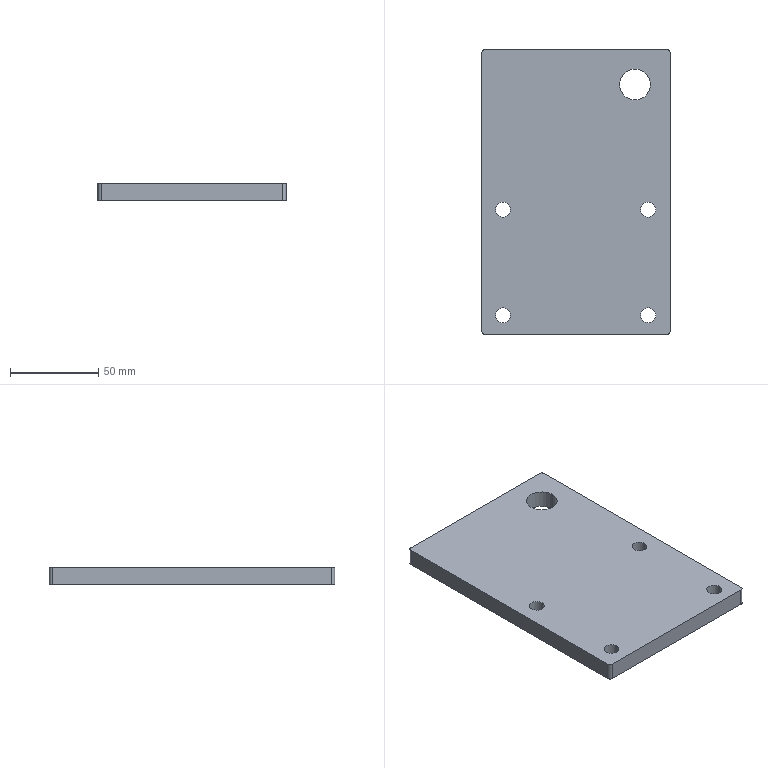Part | SolidWorks | features HoleWzd 2, Extrusion 1, Fillet 1, LPattern 1 | 1 solid | 20 faces | box 107 x 162 x 10 mm | volume 168631 mm3 | cylinder 14 | plane 6 | commonest cylinder face diameters 8.5 x8 4 x4 17.5 x2
STEP:
#1=CARTESIAN_POINT('',(36.75,-70.,-5.));
#2=VERTEX_POINT('',#1);
#3=CARTESIAN_POINT('',(45.25,-70.,-5.));
#4=VERTEX_POINT('',#3);
#5=CARTESIAN_POINT('',(41.,-70.,-5.));
#6=DIRECTION('',(0.,0.,1.));
#7=DIRECTION('',(1.,0.,0.));
#8=AXIS2_PLACEMENT_3D('',#5,#6,#7);
#9=CIRCLE('',#8,4.25);
#10=EDGE_CURVE('',#2,#4,#9,.T.);
#11=ORIENTED_EDGE('',*,*,#10,.F.);
#12=CARTESIAN_POINT('',(36.75,-70.,5.));
#13=VERTEX_POINT('',#12);
#14=CARTESIAN_POINT('',(36.75,-70.,5.));
#15=DIRECTION('',(0.,0.,1.));
#16=VECTOR('',#15,1000.);
#17=LINE('',#14,#16);
#18=EDGE_CURVE('',#2,#13,#17,.T.);
#19=ORIENTED_EDGE('',*,*,#18,.T.);
#20=CARTESIAN_POINT('',(45.25,-70.,5.));
#21=VERTEX_POINT('',#20);
#22=CARTESIAN_POINT('',(41.,-70.,5.));
#23=DIRECTION('',(0.,0.,1.));
#24=DIRECTION('',(1.,0.,0.));
#25=AXIS2_PLACEMENT_3D('',#22,#23,#24);
#26=CIRCLE('',#25,4.25);
#27=EDGE_CURVE('',#13,#21,#26,.T.);
#28=ORIENTED_EDGE('',*,*,#27,.T.);
#29=CARTESIAN_POINT('',(45.25,-70.,5.));
#30=DIRECTION('',(0.,0.,1.));
#31=VECTOR('',#30,1000.);
#32=LINE('',#29,#31);
#33=EDGE_CURVE('',#4,#21,#32,.T.);
#34=ORIENTED_EDGE('',*,*,#33,.F.);
#35=EDGE_LOOP('',(#11,#19,#28,#34));
#36=FACE_OUTER_BOUND('',#35,.T.);
#37=CARTESIAN_POINT('',(41.,-70.,5.));
#38=DIRECTION('',(0.,0.,1.));
#39=DIRECTION('',(1.,0.,0.));
#40=AXIS2_PLACEMENT_3D('',#37,#38,#39);
#41=CYLINDRICAL_SURFACE('',#40,4.25);
#42=ADVANCED_FACE('',(#36),#41,.F.);
#43=CARTESIAN_POINT('',(-45.75,-70.,-5.));
#44=VERTEX_POINT('',#43);
#45=CARTESIAN_POINT('',(-37.25,-70.,-5.));
#46=VERTEX_POINT('',#45);
#47=CARTESIAN_POINT('',(-41.5,-70.,-5.));
#48=DIRECTION('',(0.,0.,1.));
#49=DIRECTION('',(1.,0.,0.));
#50=AXIS2_PLACEMENT_3D('',#47,#48,#49);
#51=CIRCLE('',#50,4.25);
#52=EDGE_CURVE('',#44,#46,#51,.T.);
#53=ORIENTED_EDGE('',*,*,#52,.F.);
#54=CARTESIAN_POINT('',(-45.75,-70.,5.));
#55=VERTEX_POINT('',#54);
#56=CARTESIAN_POINT('',(-45.75,-70.,5.));
#57=DIRECTION('',(0.,0.,1.));
#58=VECTOR('',#57,1000.);
#59=LINE('',#56,#58);
#60=EDGE_CURVE('',#44,#55,#59,.T.);
#61=ORIENTED_EDGE('',*,*,#60,.T.);
#62=CARTESIAN_POINT('',(-37.25,-70.,5.));
#63=VERTEX_POINT('',#62);
#64=CARTESIAN_POINT('',(-41.5,-70.,5.));
#65=DIRECTION('',(0.,0.,1.));
#66=DIRECTION('',(1.,0.,0.));
#67=AXIS2_PLACEMENT_3D('',#64,#65,#66);
#68=CIRCLE('',#67,4.25);
#69=EDGE_CURVE('',#55,#63,#68,.T.);
#70=ORIENTED_EDGE('',*,*,#69,.T.);
#71=CARTESIAN_POINT('',(-37.25,-70.,5.));
#72=DIRECTION('',(0.,0.,1.));
#73=VECTOR('',#72,1000.);
#74=LINE('',#71,#73);
#75=EDGE_CURVE('',#46,#63,#74,.T.);
#76=ORIENTED_EDGE('',*,*,#75,.F.);
#77=EDGE_LOOP('',(#53,#61,#70,#76));
#78=FACE_OUTER_BOUND('',#77,.T.);
#79=CARTESIAN_POINT('',(-41.5,-70.,5.));
#80=DIRECTION('',(0.,0.,1.));
#81=DIRECTION('',(1.,0.,0.));
#82=AXIS2_PLACEMENT_3D('',#79,#80,#81);
#83=CYLINDRICAL_SURFACE('',#82,4.25);
#84=ADVANCED_FACE('',(#78),#83,.F.);
#85=CARTESIAN_POINT('',(24.75,61.,-5.));
#86=VERTEX_POINT('',#85);
#87=CARTESIAN_POINT('',(42.25,61.,-5.));
#88=VERTEX_POINT('',#87);
#89=CARTESIAN_POINT('',(33.5,61.,-5.));
#90=DIRECTION('',(0.,0.,1.));
#91=DIRECTION('',(1.,0.,0.));
#92=AXIS2_PLACEMENT_3D('',#89,#90,#91);
#93=CIRCLE('',#92,8.75);
#94=EDGE_CURVE('',#86,#88,#93,.T.);
#95=ORIENTED_EDGE('',*,*,#94,.F.);
#96=CARTESIAN_POINT('',(24.75,61.,5.));
#97=VERTEX_POINT('',#96);
#98=CARTESIAN_POINT('',(24.75,61.,5.));
#99=DIRECTION('',(0.,0.,1.));
#100=VECTOR('',#99,1000.);
#101=LINE('',#98,#100);
#102=EDGE_CURVE('',#86,#97,#101,.T.);
#103=ORIENTED_EDGE('',*,*,#102,.T.);
#104=CARTESIAN_POINT('',(42.25,61.,5.));
#105=VERTEX_POINT('',#104);
#106=CARTESIAN_POINT('',(33.5,61.,5.));
#107=DIRECTION('',(0.,0.,1.));
#108=DIRECTION('',(1.,0.,0.));
#109=AXIS2_PLACEMENT_3D('',#106,#107,#108);
#110=CIRCLE('',#109,8.75);
#111=EDGE_CURVE('',#97,#105,#110,.T.);
#112=ORIENTED_EDGE('',*,*,#111,.T.);
#113=CARTESIAN_POINT('',(42.25,61.,5.));
#114=DIRECTION('',(0.,0.,1.));
#115=VECTOR('',#114,1000.);
#116=LINE('',#113,#115);
#117=EDGE_CURVE('',#88,#105,#116,.T.);
#118=ORIENTED_EDGE('',*,*,#117,.F.);
#119=EDGE_LOOP('',(#95,#103,#112,#118));
#120=FACE_OUTER_BOUND('',#119,.T.);
#121=CARTESIAN_POINT('',(33.5,61.,5.));
#122=DIRECTION('',(0.,0.,1.));
#123=DIRECTION('',(1.,0.,0.));
#124=AXIS2_PLACEMENT_3D('',#121,#122,#123);
#125=CYLINDRICAL_SURFACE('',#124,8.75);
#126=ADVANCED_FACE('',(#120),#125,.F.);
#127=CARTESIAN_POINT('',(-45.75,-10.,-5.));
#128=VERTEX_POINT('',#127);
#129=CARTESIAN_POINT('',(-37.25,-10.,-5.));
#130=VERTEX_POINT('',#129);
#131=CARTESIAN_POINT('',(-41.5,-10.,-5.));
#132=DIRECTION('',(0.,0.,1.));
#133=DIRECTION('',(1.,0.,0.));
#134=AXIS2_PLACEMENT_3D('',#131,#132,#133);
#135=CIRCLE('',#134,4.25);
#136=EDGE_CURVE('',#128,#130,#135,.T.);
#137=ORIENTED_EDGE('',*,*,#136,.F.);
#138=CARTESIAN_POINT('',(-45.75,-10.,5.));
#139=VERTEX_POINT('',#138);
#140=CARTESIAN_POINT('',(-45.75,-10.,5.));
#141=DIRECTION('',(0.,0.,1.));
#142=VECTOR('',#141,1000.);
#143=LINE('',#140,#142);
#144=EDGE_CURVE('',#128,#139,#143,.T.);
#145=ORIENTED_EDGE('',*,*,#144,.T.);
#146=CARTESIAN_POINT('',(-37.25,-10.,5.));
#147=VERTEX_POINT('',#146);
#148=CARTESIAN_POINT('',(-41.5,-10.,5.));
#149=DIRECTION('',(0.,0.,1.));
#150=DIRECTION('',(1.,0.,0.));
#151=AXIS2_PLACEMENT_3D('',#148,#149,#150);
#152=CIRCLE('',#151,4.25);
#153=EDGE_CURVE('',#139,#147,#152,.T.);
#154=ORIENTED_EDGE('',*,*,#153,.T.);
#155=CARTESIAN_POINT('',(-37.25,-10.,5.));
#156=DIRECTION('',(0.,0.,1.));
#157=VECTOR('',#156,1000.);
#158=LINE('',#155,#157);
#159=EDGE_CURVE('',#130,#147,#158,.T.);
#160=ORIENTED_EDGE('',*,*,#159,.F.);
#161=EDGE_LOOP('',(#137,#145,#154,#160));
#162=FACE_OUTER_BOUND('',#161,.T.);
#163=CARTESIAN_POINT('',(-41.5,-10.,5.));
#164=DIRECTION('',(0.,0.,1.));
#165=DIRECTION('',(1.,0.,0.));
#166=AXIS2_PLACEMENT_3D('',#163,#164,#165);
#167=CYLINDRICAL_SURFACE('',#166,4.25);
#168=ADVANCED_FACE('',(#162),#167,.F.);
#169=CARTESIAN_POINT('',(36.75,-10.,-5.));
#170=VERTEX_POINT('',#169);
#171=CARTESIAN_POINT('',(45.25,-10.,-5.));
#172=VERTEX_POINT('',#171);
#173=CARTESIAN_POINT('',(41.,-10.,-5.));
#174=DIRECTION('',(0.,0.,1.));
#175=DIRECTION('',(1.,0.,0.));
#176=AXIS2_PLACEMENT_3D('',#173,#174,#175);
#177=CIRCLE('',#176,4.25);
#178=EDGE_CURVE('',#170,#172,#177,.T.);
#179=ORIENTED_EDGE('',*,*,#178,.F.);
#180=CARTESIAN_POINT('',(36.75,-10.,5.));
#181=VERTEX_POINT('',#180);
#182=CARTESIAN_POINT('',(36.75,-10.,5.));
#183=DIRECTION('',(0.,0.,1.));
#184=VECTOR('',#183,1000.);
#185=LINE('',#182,#184);
#186=EDGE_CURVE('',#170,#181,#185,.T.);
#187=ORIENTED_EDGE('',*,*,#186,.T.);
#188=CARTESIAN_POINT('',(45.25,-10.,5.));
#189=VERTEX_POINT('',#188);
#190=CARTESIAN_POINT('',(41.,-10.,5.));
#191=DIRECTION('',(0.,0.,1.));
#192=DIRECTION('',(1.,0.,0.));
#193=AXIS2_PLACEMENT_3D('',#190,#191,#192);
#194=CIRCLE('',#193,4.25);
#195=EDGE_CURVE('',#181,#189,#194,.T.);
#196=ORIENTED_EDGE('',*,*,#195,.T.);
#197=CARTESIAN_POINT('',(45.25,-10.,5.));
#198=DIRECTION('',(0.,0.,1.));
#199=VECTOR('',#198,1000.);
#200=LINE('',#197,#199);
#201=EDGE_CURVE('',#172,#189,#200,.T.);
#202=ORIENTED_EDGE('',*,*,#201,.F.);
#203=EDGE_LOOP('',(#179,#187,#196,#202));
#204=FACE_OUTER_BOUND('',#203,.T.);
#205=CARTESIAN_POINT('',(41.,-10.,5.));
#206=DIRECTION('',(0.,0.,1.));
#207=DIRECTION('',(1.,0.,0.));
#208=AXIS2_PLACEMENT_3D('',#205,#206,#207);
#209=CYLINDRICAL_SURFACE('',#208,4.25);
#210=ADVANCED_FACE('',(#204),#209,.F.);
#211=ORIENTED_EDGE('',*,*,#186,.F.);
#212=CARTESIAN_POINT('',(41.,-10.,-5.));
#213=DIRECTION('',(0.,0.,1.));
#214=DIRECTION('',(1.,0.,0.));
#215=AXIS2_PLACEMENT_3D('',#212,#213,#214);
#216=CIRCLE('',#215,4.25);
#217=EDGE_CURVE('',#172,#170,#216,.T.);
#218=ORIENTED_EDGE('',*,*,#217,.F.);
#219=ORIENTED_EDGE('',*,*,#201,.T.);
#220=CARTESIAN_POINT('',(41.,-10.,5.));
#221=DIRECTION('',(0.,0.,1.));
#222=DIRECTION('',(1.,0.,0.));
#223=AXIS2_PLACEMENT_3D('',#220,#221,#222);
#224=CIRCLE('',#223,4.25);
#225=EDGE_CURVE('',#189,#181,#224,.T.);
#226=ORIENTED_EDGE('',*,*,#225,.T.);
#227=EDGE_LOOP('',(#211,#218,#219,#226));
#228=FACE_OUTER_BOUND('',#227,.T.);
#229=CARTESIAN_POINT('',(41.,-10.,5.));
#230=DIRECTION('',(0.,0.,1.));
#231=DIRECTION('',(1.,0.,0.));
#232=AXIS2_PLACEMENT_3D('',#229,#230,#231);
#233=CYLINDRICAL_SURFACE('',#232,4.25);
#234=ADVANCED_FACE('',(#228),#233,.F.);
#235=ORIENTED_EDGE('',*,*,#144,.F.);
#236=CARTESIAN_POINT('',(-41.5,-10.,-5.));
#237=DIRECTION('',(0.,0.,1.));
#238=DIRECTION('',(1.,0.,0.));
#239=AXIS2_PLACEMENT_3D('',#236,#237,#238);
#240=CIRCLE('',#239,4.25);
#241=EDGE_CURVE('',#130,#128,#240,.T.);
#242=ORIENTED_EDGE('',*,*,#241,.F.);
#243=ORIENTED_EDGE('',*,*,#159,.T.);
#244=CARTESIAN_POINT('',(-41.5,-10.,5.));
#245=DIRECTION('',(0.,0.,1.));
#246=DIRECTION('',(1.,0.,0.));
#247=AXIS2_PLACEMENT_3D('',#244,#245,#246);
#248=CIRCLE('',#247,4.25);
#249=EDGE_CURVE('',#147,#139,#248,.T.);
#250=ORIENTED_EDGE('',*,*,#249,.T.);
#251=EDGE_LOOP('',(#235,#242,#243,#250));
#252=FACE_OUTER_BOUND('',#251,.T.);
#253=CARTESIAN_POINT('',(-41.5,-10.,5.));
#254=DIRECTION('',(0.,0.,1.));
#255=DIRECTION('',(1.,0.,0.));
#256=AXIS2_PLACEMENT_3D('',#253,#254,#255);
#257=CYLINDRICAL_SURFACE('',#256,4.25);
#258=ADVANCED_FACE('',(#252),#257,.F.);
#259=CARTESIAN_POINT('',(41.,-70.,-5.));
#260=DIRECTION('',(0.,0.,1.));
#261=DIRECTION('',(1.,0.,0.));
#262=AXIS2_PLACEMENT_3D('',#259,#260,#261);
#263=CIRCLE('',#262,4.25);
#264=EDGE_CURVE('',#4,#2,#263,.T.);
#265=ORIENTED_EDGE('',*,*,#264,.T.);
#266=ORIENTED_EDGE('',*,*,#10,.T.);
#267=EDGE_LOOP('',(#265,#266));
#268=FACE_BOUND('',#267,.T.);
#269=CARTESIAN_POINT('',(-51.5,-81.,-5.));
#270=VERTEX_POINT('',#269);
#271=CARTESIAN_POINT('',(51.5,-81.,-5.));
#272=VERTEX_POINT('',#271);
#273=CARTESIAN_POINT('',(-53.5,-81.,-5.));
#274=DIRECTION('',(1.,0.,0.));
#275=VECTOR('',#274,1000.);
#276=LINE('',#273,#275);
#277=EDGE_CURVE('',#270,#272,#276,.T.);
#278=ORIENTED_EDGE('',*,*,#277,.F.);
#279=CARTESIAN_POINT('',(-53.5,-79.,-5.));
#280=VERTEX_POINT('',#279);
#281=CARTESIAN_POINT('',(-51.5,-79.,-5.));
#282=DIRECTION('',(0.,0.,-1.));
#283=DIRECTION('',(-1.,0.,0.));
#284=AXIS2_PLACEMENT_3D('',#281,#282,#283);
#285=CIRCLE('',#284,2.);
#286=EDGE_CURVE('',#270,#280,#285,.T.);
#287=ORIENTED_EDGE('',*,*,#286,.T.);
#288=CARTESIAN_POINT('',(-53.5,79.,-5.));
#289=VERTEX_POINT('',#288);
#290=CARTESIAN_POINT('',(-53.5,-81.,-5.));
#291=DIRECTION('',(0.,-1.,0.));
#292=VECTOR('',#291,1000.);
#293=LINE('',#290,#292);
#294=EDGE_CURVE('',#289,#280,#293,.T.);
#295=ORIENTED_EDGE('',*,*,#294,.F.);
#296=CARTESIAN_POINT('',(-51.5,81.,-5.));
#297=VERTEX_POINT('',#296);
#298=CARTESIAN_POINT('',(-51.5,79.,-5.));
#299=DIRECTION('',(0.,0.,-1.));
#300=DIRECTION('',(-1.,0.,0.));
#301=AXIS2_PLACEMENT_3D('',#298,#299,#300);
#302=CIRCLE('',#301,2.);
#303=EDGE_CURVE('',#289,#297,#302,.T.);
#304=ORIENTED_EDGE('',*,*,#303,.T.);
#305=CARTESIAN_POINT('',(51.5,81.,-5.));
#306=VERTEX_POINT('',#305);
#307=CARTESIAN_POINT('',(-53.5,81.,-5.));
#308=DIRECTION('',(-1.,0.,0.));
#309=VECTOR('',#308,1000.);
#310=LINE('',#307,#309);
#311=EDGE_CURVE('',#306,#297,#310,.T.);
#312=ORIENTED_EDGE('',*,*,#311,.F.);
#313=CARTESIAN_POINT('',(53.5,79.,-5.));
#314=VERTEX_POINT('',#313);
#315=CARTESIAN_POINT('',(51.5,79.,-5.));
#316=DIRECTION('',(0.,0.,-1.));
#317=DIRECTION('',(-1.,0.,0.));
#318=AXIS2_PLACEMENT_3D('',#315,#316,#317);
#319=CIRCLE('',#318,2.);
#320=EDGE_CURVE('',#306,#314,#319,.T.);
#321=ORIENTED_EDGE('',*,*,#320,.T.);
#322=CARTESIAN_POINT('',(53.5,-79.,-5.));
#323=VERTEX_POINT('',#322);
#324=CARTESIAN_POINT('',(53.5,-81.,-5.));
#325=DIRECTION('',(0.,1.,0.));
#326=VECTOR('',#325,1000.);
#327=LINE('',#324,#326);
#328=EDGE_CURVE('',#323,#314,#327,.T.);
#329=ORIENTED_EDGE('',*,*,#328,.F.);
#330=CARTESIAN_POINT('',(51.5,-79.,-5.));
#331=DIRECTION('',(0.,0.,-1.));
#332=DIRECTION('',(-1.,0.,0.));
#333=AXIS2_PLACEMENT_3D('',#330,#331,#332);
#334=CIRCLE('',#333,2.);
#335=EDGE_CURVE('',#323,#272,#334,.T.);
#336=ORIENTED_EDGE('',*,*,#335,.T.);
#337=EDGE_LOOP('',(#278,#287,#295,#304,#312,#321,#329,#336));
#338=FACE_OUTER_BOUND('',#337,.T.);
#339=CARTESIAN_POINT('',(33.5,61.,-5.));
#340=DIRECTION('',(0.,0.,1.));
#341=DIRECTION('',(1.,0.,0.));
#342=AXIS2_PLACEMENT_3D('',#339,#340,#341);
#343=CIRCLE('',#342,8.75);
#344=EDGE_CURVE('',#88,#86,#343,.T.);
#345=ORIENTED_EDGE('',*,*,#344,.T.);
#346=ORIENTED_EDGE('',*,*,#94,.T.);
#347=EDGE_LOOP('',(#345,#346));
#348=FACE_BOUND('',#347,.T.);
#349=CARTESIAN_POINT('',(-41.5,-70.,-5.));
#350=DIRECTION('',(0.,0.,1.));
#351=DIRECTION('',(1.,0.,0.));
#352=AXIS2_PLACEMENT_3D('',#349,#350,#351);
#353=CIRCLE('',#352,4.25);
#354=EDGE_CURVE('',#46,#44,#353,.T.);
#355=ORIENTED_EDGE('',*,*,#354,.T.);
#356=ORIENTED_EDGE('',*,*,#52,.T.);
#357=EDGE_LOOP('',(#355,#356));
#358=FACE_BOUND('',#357,.T.);
#359=ORIENTED_EDGE('',*,*,#241,.T.);
#360=ORIENTED_EDGE('',*,*,#136,.T.);
#361=EDGE_LOOP('',(#359,#360));
#362=FACE_BOUND('',#361,.T.);
#363=ORIENTED_EDGE('',*,*,#217,.T.);
#364=ORIENTED_EDGE('',*,*,#178,.T.);
#365=EDGE_LOOP('',(#363,#364));
#366=FACE_BOUND('',#365,.T.);
#367=CARTESIAN_POINT('',(0.,0.,-5.));
#368=DIRECTION('',(0.,0.,-1.));
#369=DIRECTION('',(-1.,0.,0.));
#370=AXIS2_PLACEMENT_3D('',#367,#368,#369);
#371=PLANE('',#370);
#372=ADVANCED_FACE('',(#268,#338,#348,#358,#362,#366),#371,.T.);
#373=CARTESIAN_POINT('',(53.5,-79.,5.));
#374=VERTEX_POINT('',#373);
#375=CARTESIAN_POINT('',(53.5,79.,5.));
#376=VERTEX_POINT('',#375);
#377=CARTESIAN_POINT('',(53.5,-81.,5.));
#378=DIRECTION('',(0.,1.,0.));
#379=VECTOR('',#378,1000.);
#380=LINE('',#377,#379);
#381=EDGE_CURVE('',#374,#376,#380,.T.);
#382=ORIENTED_EDGE('',*,*,#381,.F.);
#383=CARTESIAN_POINT('',(53.5,-79.,5.));
#384=DIRECTION('',(0.,0.,-1.));
#385=VECTOR('',#384,1000.);
#386=LINE('',#383,#385);
#387=EDGE_CURVE('',#374,#323,#386,.T.);
#388=ORIENTED_EDGE('',*,*,#387,.T.);
#389=ORIENTED_EDGE('',*,*,#328,.T.);
#390=CARTESIAN_POINT('',(53.5,79.,5.));
#391=DIRECTION('',(0.,0.,1.));
#392=VECTOR('',#391,1000.);
#393=LINE('',#390,#392);
#394=EDGE_CURVE('',#314,#376,#393,.T.);
#395=ORIENTED_EDGE('',*,*,#394,.T.);
#396=EDGE_LOOP('',(#382,#388,#389,#395));
#397=FACE_OUTER_BOUND('',#396,.T.);
#398=CARTESIAN_POINT('',(53.5,-81.,5.));
#399=DIRECTION('',(-1.,0.,0.));
#400=DIRECTION('',(0.,0.,1.));
#401=AXIS2_PLACEMENT_3D('',#398,#399,#400);
#402=PLANE('',#401);
#403=ADVANCED_FACE('',(#397),#402,.F.);
#404=CARTESIAN_POINT('',(51.5,81.,5.));
#405=VERTEX_POINT('',#404);
#406=CARTESIAN_POINT('',(-51.5,81.,5.));
#407=VERTEX_POINT('',#406);
#408=CARTESIAN_POINT('',(-53.5,81.,5.));
#409=DIRECTION('',(-1.,0.,0.));
#410=VECTOR('',#409,1000.);
#411=LINE('',#408,#410);
#412=EDGE_CURVE('',#405,#407,#411,.T.);
#413=ORIENTED_EDGE('',*,*,#412,.F.);
#414=CARTESIAN_POINT('',(51.5,81.,5.));
#415=DIRECTION('',(0.,0.,-1.));
#416=VECTOR('',#415,1000.);
#417=LINE('',#414,#416);
#418=EDGE_CURVE('',#405,#306,#417,.T.);
#419=ORIENTED_EDGE('',*,*,#418,.T.);
#420=ORIENTED_EDGE('',*,*,#311,.T.);
#421=CARTESIAN_POINT('',(-51.5,81.,5.));
#422=DIRECTION('',(0.,0.,1.));
#423=VECTOR('',#422,1000.);
#424=LINE('',#421,#423);
#425=EDGE_CURVE('',#297,#407,#424,.T.);
#426=ORIENTED_EDGE('',*,*,#425,.T.);
#427=EDGE_LOOP('',(#413,#419,#420,#426));
#428=FACE_OUTER_BOUND('',#427,.T.);
#429=CARTESIAN_POINT('',(-53.5,81.,5.));
#430=DIRECTION('',(0.,-1.,0.));
#431=DIRECTION('',(0.,0.,-1.));
#432=AXIS2_PLACEMENT_3D('',#429,#430,#431);
#433=PLANE('',#432);
#434=ADVANCED_FACE('',(#428),#433,.F.);
#435=ORIENTED_EDGE('',*,*,#294,.T.);
#436=CARTESIAN_POINT('',(-53.5,-79.,5.));
#437=VERTEX_POINT('',#436);
#438=CARTESIAN_POINT('',(-53.5,-79.,5.));
#439=DIRECTION('',(0.,0.,1.));
#440=VECTOR('',#439,1000.);
#441=LINE('',#438,#440);
#442=EDGE_CURVE('',#280,#437,#441,.T.);
#443=ORIENTED_EDGE('',*,*,#442,.T.);
#444=CARTESIAN_POINT('',(-53.5,79.,5.));
#445=VERTEX_POINT('',#444);
#446=CARTESIAN_POINT('',(-53.5,-81.,5.));
#447=DIRECTION('',(0.,-1.,0.));
#448=VECTOR('',#447,1000.);
#449=LINE('',#446,#448);
#450=EDGE_CURVE('',#445,#437,#449,.T.);
#451=ORIENTED_EDGE('',*,*,#450,.F.);
#452=CARTESIAN_POINT('',(-53.5,79.,5.));
#453=DIRECTION('',(0.,0.,-1.));
#454=VECTOR('',#453,1000.);
#455=LINE('',#452,#454);
#456=EDGE_CURVE('',#445,#289,#455,.T.);
#457=ORIENTED_EDGE('',*,*,#456,.T.);
#458=EDGE_LOOP('',(#435,#443,#451,#457));
#459=FACE_OUTER_BOUND('',#458,.T.);
#460=CARTESIAN_POINT('',(-53.5,-81.,5.));
#461=DIRECTION('',(1.,0.,0.));
#462=DIRECTION('',(0.,0.,-1.));
#463=AXIS2_PLACEMENT_3D('',#460,#461,#462);
#464=PLANE('',#463);
#465=ADVANCED_FACE('',(#459),#464,.F.);
#466=CARTESIAN_POINT('',(-51.5,-81.,5.));
#467=VERTEX_POINT('',#466);
#468=CARTESIAN_POINT('',(51.5,-81.,5.));
#469=VERTEX_POINT('',#468);
#470=CARTESIAN_POINT('',(-53.5,-81.,5.));
#471=DIRECTION('',(1.,0.,0.));
#472=VECTOR('',#471,1000.);
#473=LINE('',#470,#472);
#474=EDGE_CURVE('',#467,#469,#473,.T.);
#475=ORIENTED_EDGE('',*,*,#474,.F.);
#476=CARTESIAN_POINT('',(-51.5,-81.,5.));
#477=DIRECTION('',(0.,0.,-1.));
#478=VECTOR('',#477,1000.);
#479=LINE('',#476,#478);
#480=EDGE_CURVE('',#467,#270,#479,.T.);
#481=ORIENTED_EDGE('',*,*,#480,.T.);
#482=ORIENTED_EDGE('',*,*,#277,.T.);
#483=CARTESIAN_POINT('',(51.5,-81.,5.));
#484=DIRECTION('',(0.,0.,1.));
#485=VECTOR('',#484,1000.);
#486=LINE('',#483,#485);
#487=EDGE_CURVE('',#272,#469,#486,.T.);
#488=ORIENTED_EDGE('',*,*,#487,.T.);
#489=EDGE_LOOP('',(#475,#481,#482,#488));
#490=FACE_OUTER_BOUND('',#489,.T.);
#491=CARTESIAN_POINT('',(-53.5,-81.,5.));
#492=DIRECTION('',(0.,1.,0.));
#493=DIRECTION('',(0.,0.,1.));
#494=AXIS2_PLACEMENT_3D('',#491,#492,#493);
#495=PLANE('',#494);
#496=ADVANCED_FACE('',(#490),#495,.F.);
#497=CARTESIAN_POINT('',(41.,-70.,5.));
#498=DIRECTION('',(0.,0.,1.));
#499=DIRECTION('',(1.,0.,0.));
#500=AXIS2_PLACEMENT_3D('',#497,#498,#499);
#501=CIRCLE('',#500,4.25);
#502=EDGE_CURVE('',#21,#13,#501,.T.);
#503=ORIENTED_EDGE('',*,*,#502,.F.);
#504=ORIENTED_EDGE('',*,*,#27,.F.);
#505=EDGE_LOOP('',(#503,#504));
#506=FACE_BOUND('',#505,.T.);
#507=CARTESIAN_POINT('',(-41.5,-70.,5.));
#508=DIRECTION('',(0.,0.,1.));
#509=DIRECTION('',(1.,0.,0.));
#510=AXIS2_PLACEMENT_3D('',#507,#508,#509);
#511=CIRCLE('',#510,4.25);
#512=EDGE_CURVE('',#63,#55,#511,.T.);
#513=ORIENTED_EDGE('',*,*,#512,.F.);
#514=ORIENTED_EDGE('',*,*,#69,.F.);
#515=EDGE_LOOP('',(#513,#514));
#516=FACE_BOUND('',#515,.T.);
#517=CARTESIAN_POINT('',(33.5,61.,5.));
#518=DIRECTION('',(0.,0.,1.));
#519=DIRECTION('',(1.,0.,0.));
#520=AXIS2_PLACEMENT_3D('',#517,#518,#519);
#521=CIRCLE('',#520,8.75);
#522=EDGE_CURVE('',#105,#97,#521,.T.);
#523=ORIENTED_EDGE('',*,*,#522,.F.);
#524=ORIENTED_EDGE('',*,*,#111,.F.);
#525=EDGE_LOOP('',(#523,#524));
#526=FACE_BOUND('',#525,.T.);
#527=ORIENTED_EDGE('',*,*,#450,.T.);
#528=CARTESIAN_POINT('',(-51.5,-79.,5.));
#529=DIRECTION('',(0.,0.,1.));
#530=DIRECTION('',(-1.,0.,0.));
#531=AXIS2_PLACEMENT_3D('',#528,#529,#530);
#532=CIRCLE('',#531,2.);
#533=EDGE_CURVE('',#437,#467,#532,.T.);
#534=ORIENTED_EDGE('',*,*,#533,.T.);
#535=ORIENTED_EDGE('',*,*,#474,.T.);
#536=CARTESIAN_POINT('',(51.5,-79.,5.));
#537=DIRECTION('',(0.,0.,1.));
#538=DIRECTION('',(-1.,0.,0.));
#539=AXIS2_PLACEMENT_3D('',#536,#537,#538);
#540=CIRCLE('',#539,2.);
#541=EDGE_CURVE('',#469,#374,#540,.T.);
#542=ORIENTED_EDGE('',*,*,#541,.T.);
#543=ORIENTED_EDGE('',*,*,#381,.T.);
#544=CARTESIAN_POINT('',(51.5,79.,5.));
#545=DIRECTION('',(0.,0.,1.));
#546=DIRECTION('',(-1.,0.,0.));
#547=AXIS2_PLACEMENT_3D('',#544,#545,#546);
#548=CIRCLE('',#547,2.);
#549=EDGE_CURVE('',#376,#405,#548,.T.);
#550=ORIENTED_EDGE('',*,*,#549,.T.);
#551=ORIENTED_EDGE('',*,*,#412,.T.);
#552=CARTESIAN_POINT('',(-51.5,79.,5.));
#553=DIRECTION('',(0.,0.,1.));
#554=DIRECTION('',(-1.,0.,0.));
#555=AXIS2_PLACEMENT_3D('',#552,#553,#554);
#556=CIRCLE('',#555,2.);
#557=EDGE_CURVE('',#407,#445,#556,.T.);
#558=ORIENTED_EDGE('',*,*,#557,.T.);
#559=EDGE_LOOP('',(#527,#534,#535,#542,#543,#550,#551,#558));
#560=FACE_OUTER_BOUND('',#559,.T.);
#561=ORIENTED_EDGE('',*,*,#249,.F.);
#562=ORIENTED_EDGE('',*,*,#153,.F.);
#563=EDGE_LOOP('',(#561,#562));
#564=FACE_BOUND('',#563,.T.);
#565=ORIENTED_EDGE('',*,*,#225,.F.);
#566=ORIENTED_EDGE('',*,*,#195,.F.);
#567=EDGE_LOOP('',(#565,#566));
#568=FACE_BOUND('',#567,.T.);
#569=CARTESIAN_POINT('',(0.,0.,5.));
#570=DIRECTION('',(0.,0.,-1.));
#571=DIRECTION('',(-1.,0.,0.));
#572=AXIS2_PLACEMENT_3D('',#569,#570,#571);
#573=PLANE('',#572);
#574=ADVANCED_FACE('',(#506,#516,#526,#560,#564,#568),#573,.F.);
#575=ORIENTED_EDGE('',*,*,#102,.F.);
#576=ORIENTED_EDGE('',*,*,#344,.F.);
#577=ORIENTED_EDGE('',*,*,#117,.T.);
#578=ORIENTED_EDGE('',*,*,#522,.T.);
#579=EDGE_LOOP('',(#575,#576,#577,#578));
#580=FACE_OUTER_BOUND('',#579,.T.);
#581=CARTESIAN_POINT('',(33.5,61.,5.));
#582=DIRECTION('',(0.,0.,1.));
#583=DIRECTION('',(1.,0.,0.));
#584=AXIS2_PLACEMENT_3D('',#581,#582,#583);
#585=CYLINDRICAL_SURFACE('',#584,8.75);
#586=ADVANCED_FACE('',(#580),#585,.F.);
#587=ORIENTED_EDGE('',*,*,#533,.F.);
#588=ORIENTED_EDGE('',*,*,#442,.F.);
#589=ORIENTED_EDGE('',*,*,#286,.F.);
#590=ORIENTED_EDGE('',*,*,#480,.F.);
#591=EDGE_LOOP('',(#587,#588,#589,#590));
#592=FACE_OUTER_BOUND('',#591,.T.);
#593=CARTESIAN_POINT('',(-51.5,-79.,5.));
#594=DIRECTION('',(0.,0.,-1.));
#595=DIRECTION('',(-1.,0.,0.));
#596=AXIS2_PLACEMENT_3D('',#593,#594,#595);
#597=CYLINDRICAL_SURFACE('',#596,2.);
#598=ADVANCED_FACE('',(#592),#597,.T.);
#599=ORIENTED_EDGE('',*,*,#541,.F.);
#600=ORIENTED_EDGE('',*,*,#487,.F.);
#601=ORIENTED_EDGE('',*,*,#335,.F.);
#602=ORIENTED_EDGE('',*,*,#387,.F.);
#603=EDGE_LOOP('',(#599,#600,#601,#602));
#604=FACE_OUTER_BOUND('',#603,.T.);
#605=CARTESIAN_POINT('',(51.5,-79.,5.));
#606=DIRECTION('',(0.,0.,-1.));
#607=DIRECTION('',(-1.,0.,0.));
#608=AXIS2_PLACEMENT_3D('',#605,#606,#607);
#609=CYLINDRICAL_SURFACE('',#608,2.);
#610=ADVANCED_FACE('',(#604),#609,.T.);
#611=ORIENTED_EDGE('',*,*,#549,.F.);
#612=ORIENTED_EDGE('',*,*,#394,.F.);
#613=ORIENTED_EDGE('',*,*,#320,.F.);
#614=ORIENTED_EDGE('',*,*,#418,.F.);
#615=EDGE_LOOP('',(#611,#612,#613,#614));
#616=FACE_OUTER_BOUND('',#615,.T.);
#617=CARTESIAN_POINT('',(51.5,79.,5.));
#618=DIRECTION('',(0.,0.,-1.));
#619=DIRECTION('',(-1.,0.,0.));
#620=AXIS2_PLACEMENT_3D('',#617,#618,#619);
#621=CYLINDRICAL_SURFACE('',#620,2.);
#622=ADVANCED_FACE('',(#616),#621,.T.);
#623=ORIENTED_EDGE('',*,*,#557,.F.);
#624=ORIENTED_EDGE('',*,*,#425,.F.);
#625=ORIENTED_EDGE('',*,*,#303,.F.);
#626=ORIENTED_EDGE('',*,*,#456,.F.);
#627=EDGE_LOOP('',(#623,#624,#625,#626));
#628=FACE_OUTER_BOUND('',#627,.T.);
#629=CARTESIAN_POINT('',(-51.5,79.,5.));
#630=DIRECTION('',(0.,0.,-1.));
#631=DIRECTION('',(-1.,0.,0.));
#632=AXIS2_PLACEMENT_3D('',#629,#630,#631);
#633=CYLINDRICAL_SURFACE('',#632,2.);
#634=ADVANCED_FACE('',(#628),#633,.T.);
#635=ORIENTED_EDGE('',*,*,#60,.F.);
#636=ORIENTED_EDGE('',*,*,#354,.F.);
#637=ORIENTED_EDGE('',*,*,#75,.T.);
#638=ORIENTED_EDGE('',*,*,#512,.T.);
#639=EDGE_LOOP('',(#635,#636,#637,#638));
#640=FACE_OUTER_BOUND('',#639,.T.);
#641=CARTESIAN_POINT('',(-41.5,-70.,5.));
#642=DIRECTION('',(0.,0.,1.));
#643=DIRECTION('',(1.,0.,0.));
#644=AXIS2_PLACEMENT_3D('',#641,#642,#643);
#645=CYLINDRICAL_SURFACE('',#644,4.25);
#646=ADVANCED_FACE('',(#640),#645,.F.);
#647=ORIENTED_EDGE('',*,*,#18,.F.);
#648=ORIENTED_EDGE('',*,*,#264,.F.);
#649=ORIENTED_EDGE('',*,*,#33,.T.);
#650=ORIENTED_EDGE('',*,*,#502,.T.);
#651=EDGE_LOOP('',(#647,#648,#649,#650));
#652=FACE_OUTER_BOUND('',#651,.T.);
#653=CARTESIAN_POINT('',(41.,-70.,5.));
#654=DIRECTION('',(0.,0.,1.));
#655=DIRECTION('',(1.,0.,0.));
#656=AXIS2_PLACEMENT_3D('',#653,#654,#655);
#657=CYLINDRICAL_SURFACE('',#656,4.25);
#658=ADVANCED_FACE('',(#652),#657,.F.);
#659=CLOSED_SHELL('',(#42,#84,#126,#168,#210,#234,#258,#372,#403,#434,#465,#496,#574,#586,#598,#610,#622,#634,#646,#658));
#660=MANIFOLD_SOLID_BREP('',#659);
#661=CARTESIAN_POINT('',(0.,0.,0.));
#662=DIRECTION('',(0.,0.,1.));
#663=DIRECTION('',(1.,0.,0.));
#664=AXIS2_PLACEMENT_3D('',#661,#662,#663);
#665=(LENGTH_UNIT()NAMED_UNIT(*)SI_UNIT(.MILLI.,.METRE.));
#666=UNCERTAINTY_MEASURE_WITH_UNIT(LENGTH_MEASURE(0.00001),#665,'','');
#667=(NAMED_UNIT(*)PLANE_ANGLE_UNIT()SI_UNIT($,.RADIAN.));
#668=(NAMED_UNIT(*)SI_UNIT($,.STERADIAN.)SOLID_ANGLE_UNIT());
#669=(GEOMETRIC_REPRESENTATION_CONTEXT(3)GLOBAL_UNCERTAINTY_ASSIGNED_CONTEXT((#666))GLOBAL_UNIT_ASSIGNED_CONTEXT((#665,#667,#668))REPRESENTATION_CONTEXT('',''));
#670=ADVANCED_BREP_SHAPE_REPRESENTATION('',(#660,#664),#669);